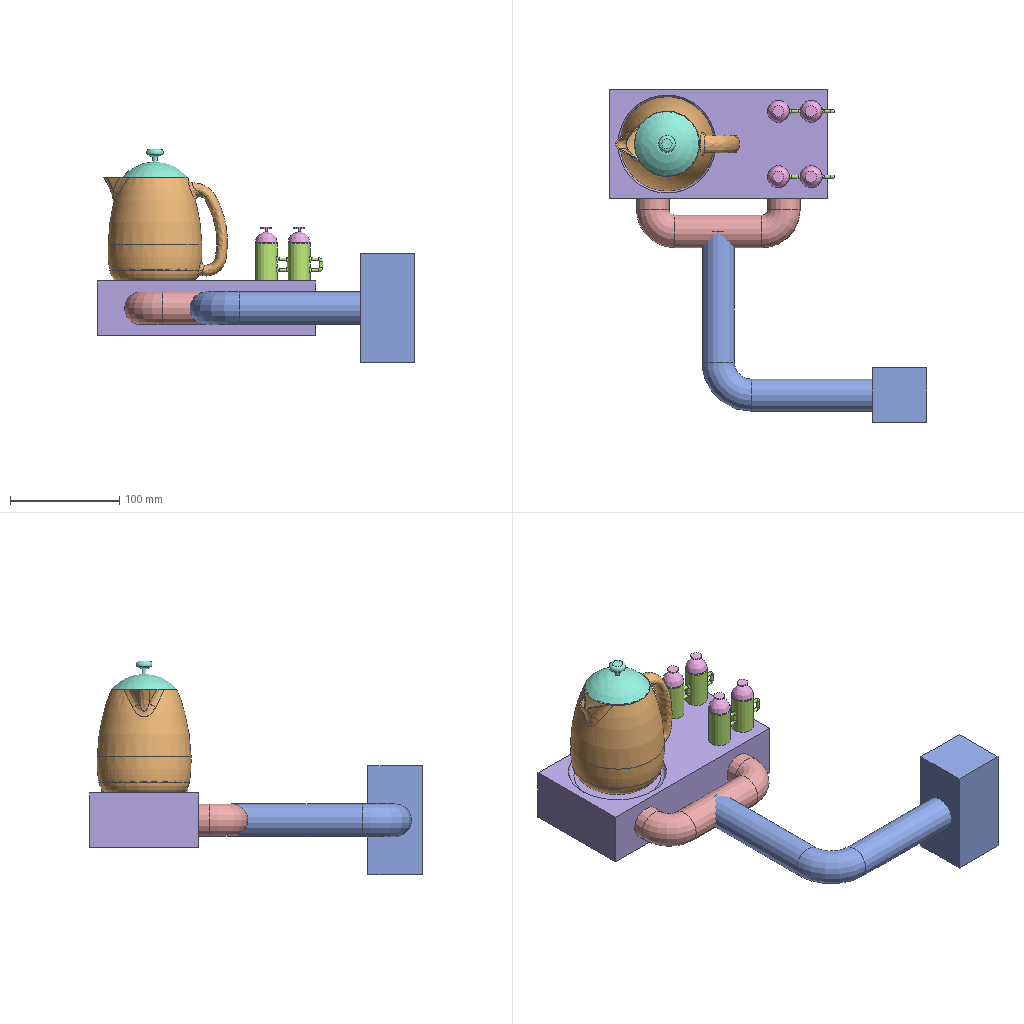Assembly | NX | 6 different items | 12 placed | box 291 x 305 x 196 mm
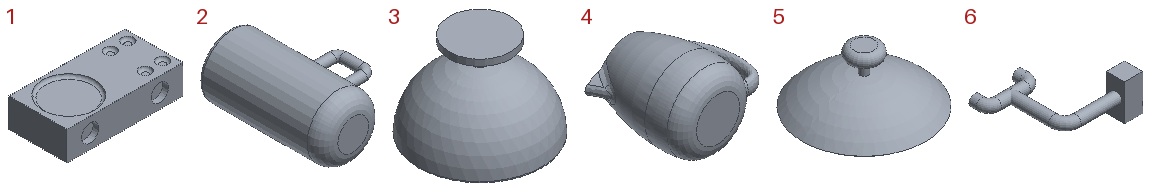Parts list (item | quantity | size | volume | features):
1 | x1 | 200 x 100 x 50 mm | 950448 mm3 | features EXTRUDE 4, DATUM_CSYS 3, BLEND 2, SKETCH 2
2 | x4 | 31.5 x 40 x 20 mm | 6808 mm3 | features BLEND 4, DATUM_CSYS 2, SWP104 2, REPLACE_FACE 1, SKETCH 1, UNITE 1
3 | x4 | 19.991 x 19.991 x 14 mm | 1108 mm3 | features DATUM_CSYS 3, SKETCH 2, BLEND 1, REPLACE_FACE 1, SHELL 1, SPHERE 1, SWP104 1, TRIM BODY 1, UNITE 1
4 | x1 | 113.54 x 100 x 86.236 mm | 41755 mm3 | features DATUM_CSYS 3, REPLACE_FACE 3, SKETCH 3, BLEND 2, OFFSET_REGION 2, SKIN 2, UNITE 2, DATUM_ON_PATH 1, SHELL 1, SWP104 1
5 | x1 | 60 x 60 x 26.776 mm | 4501 mm3 | features DATUM_CSYS 3, SKETCH 2, SWP104 2, EXTRUDE 1, SHELL 1
6 | x1 | 266 x 215 x 100 mm | 575830 mm3 | features DATUM_CSYS 3, SKETCH 2, SWP104 2, EXTRUDE 1
Mates (type | each side: item.copy, entity, surface, feature):
Touch | 4.1 face surfaceofrevolution Revolve(4) | 1.1 face surfaceofrevolution Edge Blend(5)
Touch | 4.1 face plane Revolve(4) | 1.1 face plane Extrude(3)
Touch | 5.1 face surfaceofrevolution Revolve(5) | 4.1 face surfaceofrevolution Swept(3)
Touch | 5.1 face plane Revolve(3) | 4.1 face plane Revolve(4)
Touch | 2.1 face cylinder Revolve(2) | 1.1 face surfaceofrevolution Edge Blend(6) | 2 times
Touch | 2.1 face plane Revolve(2) | 1.1 face plane Extrude(4)
Touch | 2.1 edge | 1.1 edge
Touch | 3.1 face cylinder Revolve(6) | 2.1 face cylinder Revolve(2) | 2 times
Touch | 3.1 face plane Trim Body(3) | 2.1 face plane Revolve(2) | 2 times
Touch | 6.1 face cylinder Tube(2) | 1.1 face cylinder Extrude(9)
Touch | 6.1 face plane Tube(2) | 1.1 face plane Extrude(9)